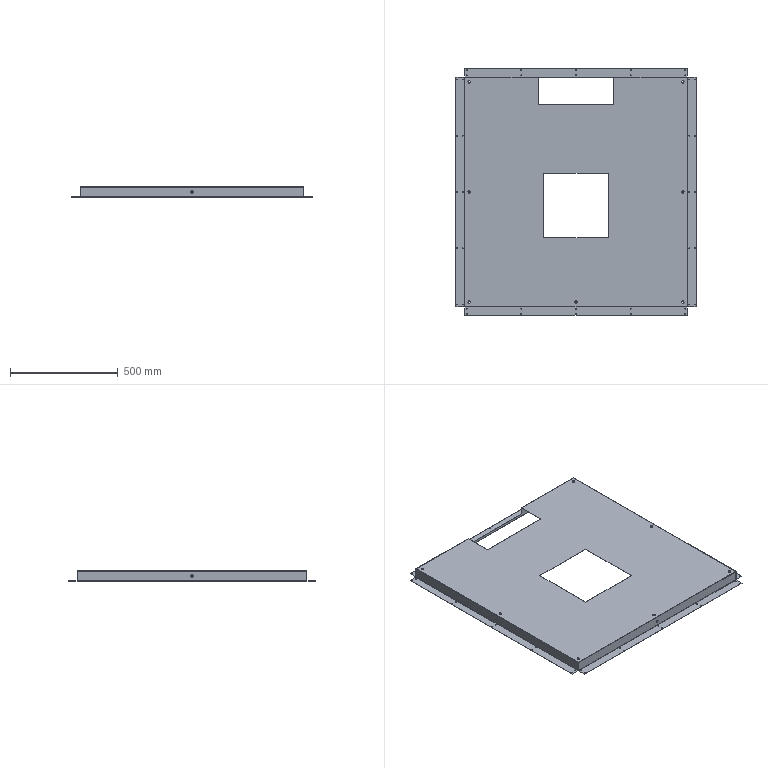Part | 1 solid | 184 faces | box 1113 x 1143 x 48 mm | volume 1312291 mm3 | cylinder 118 | plane 58 | spline 8 | commonest cylinder face diameters 4.2 x80 11 x14 0.4 x9 2.4 x9 10 x6